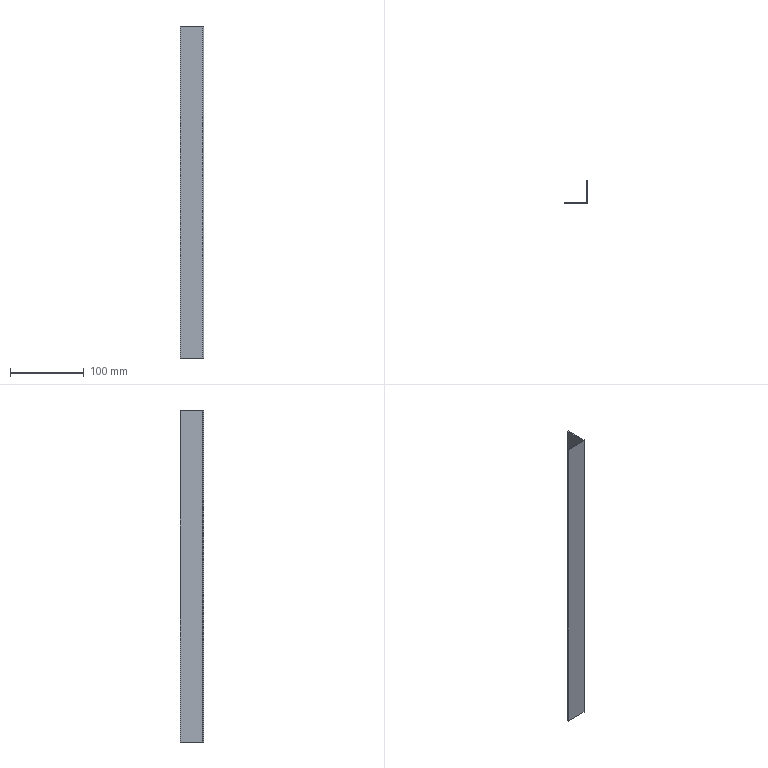Part | SolidWorks | features SplitBody 1 | 1 solid | 14 faces | box 31.5 x 31.5 x 450 mm | volume 41266 mm3 | plane 12 | cylinder 2 | commonest cylinder face diameters 0.2 x1 3.2 x1
STEP:
#1=CARTESIAN_POINT('',(-25.,30.1,185.));
#2=VERTEX_POINT('',#1);
#3=CARTESIAN_POINT('',(-23.5,30.1,185.));
#4=VERTEX_POINT('',#3);
#5=CARTESIAN_POINT('',(-25.,30.1,185.));
#6=DIRECTION('',(1.,0.,0.));
#7=VECTOR('',#6,1000.);
#8=LINE('',#5,#7);
#9=EDGE_CURVE('',#2,#4,#8,.T.);
#10=ORIENTED_EDGE('',*,*,#9,.F.);
#11=CARTESIAN_POINT('',(-25.1,30.,185.));
#12=VERTEX_POINT('',#11);
#13=CARTESIAN_POINT('',(-25.1,30.1,185.));
#14=DIRECTION('',(0.,0.,1.));
#15=DIRECTION('',(0.,1.,0.));
#16=AXIS2_PLACEMENT_3D('',#13,#14,#15);
#17=CIRCLE('',#16,0.1);
#18=EDGE_CURVE('',#12,#2,#17,.T.);
#19=ORIENTED_EDGE('',*,*,#18,.F.);
#20=CARTESIAN_POINT('',(-25.1,28.5,185.));
#21=VERTEX_POINT('',#20);
#22=CARTESIAN_POINT('',(-25.1,28.5,185.));
#23=DIRECTION('',(0.,1.,0.));
#24=VECTOR('',#23,1000.);
#25=LINE('',#22,#24);
#26=EDGE_CURVE('',#21,#12,#25,.T.);
#27=ORIENTED_EDGE('',*,*,#26,.F.);
#28=CARTESIAN_POINT('',(-25.1,30.1,185.));
#29=DIRECTION('',(0.,0.,1.));
#30=DIRECTION('',(-1.,0.,0.));
#31=AXIS2_PLACEMENT_3D('',#28,#29,#30);
#32=CIRCLE('',#31,1.6);
#33=EDGE_CURVE('',#21,#4,#32,.T.);
#34=ORIENTED_EDGE('',*,*,#33,.T.);
#35=EDGE_LOOP('',(#10,#19,#27,#34));
#36=FACE_OUTER_BOUND('',#35,.T.);
#37=CARTESIAN_POINT('',(-25.,30.1,185.));
#38=DIRECTION('',(0.,0.,1.));
#39=DIRECTION('',(0.,-1.,0.));
#40=AXIS2_PLACEMENT_3D('',#37,#38,#39);
#41=PLANE('',#40);
#42=ADVANCED_FACE('',(#36),#41,.T.);
#43=CARTESIAN_POINT('',(-25.,60.,185.));
#44=VERTEX_POINT('',#43);
#45=CARTESIAN_POINT('',(-25.,30.,185.));
#46=DIRECTION('',(0.,1.,0.));
#47=VECTOR('',#46,1000.);
#48=LINE('',#45,#47);
#49=EDGE_CURVE('',#2,#44,#48,.T.);
#50=ORIENTED_EDGE('',*,*,#49,.F.);
#51=ORIENTED_EDGE('',*,*,#9,.T.);
#52=CARTESIAN_POINT('',(-23.5,60.,185.));
#53=VERTEX_POINT('',#52);
#54=CARTESIAN_POINT('',(-23.5,30.,185.));
#55=DIRECTION('',(0.,1.,0.));
#56=VECTOR('',#55,1000.);
#57=LINE('',#54,#56);
#58=EDGE_CURVE('',#4,#53,#57,.T.);
#59=ORIENTED_EDGE('',*,*,#58,.T.);
#60=CARTESIAN_POINT('',(-23.5,60.,185.));
#61=DIRECTION('',(-1.,0.,0.));
#62=VECTOR('',#61,1000.);
#63=LINE('',#60,#62);
#64=EDGE_CURVE('',#53,#44,#63,.T.);
#65=ORIENTED_EDGE('',*,*,#64,.T.);
#66=EDGE_LOOP('',(#50,#51,#59,#65));
#67=FACE_OUTER_BOUND('',#66,.T.);
#68=CARTESIAN_POINT('',(-25.1,28.5,185.));
#69=DIRECTION('',(0.,0.,1.));
#70=DIRECTION('',(0.,-1.,0.));
#71=AXIS2_PLACEMENT_3D('',#68,#69,#70);
#72=PLANE('',#71);
#73=ADVANCED_FACE('',(#67),#72,.T.);
#74=CARTESIAN_POINT('',(-25.,60.,-265.));
#75=VERTEX_POINT('',#74);
#76=CARTESIAN_POINT('',(-25.,30.1,-265.));
#77=VERTEX_POINT('',#76);
#78=CARTESIAN_POINT('',(-25.,30.,-265.));
#79=DIRECTION('',(0.,-1.,0.));
#80=VECTOR('',#79,1000.);
#81=LINE('',#78,#80);
#82=EDGE_CURVE('',#75,#77,#81,.T.);
#83=ORIENTED_EDGE('',*,*,#82,.T.);
#84=CARTESIAN_POINT('',(-25.,30.1,-309.548));
#85=DIRECTION('',(0.,0.,1.));
#86=VECTOR('',#85,1000.);
#87=LINE('',#84,#86);
#88=EDGE_CURVE('',#77,#2,#87,.T.);
#89=ORIENTED_EDGE('',*,*,#88,.T.);
#90=ORIENTED_EDGE('',*,*,#49,.T.);
#91=CARTESIAN_POINT('',(-25.,60.,-309.548));
#92=DIRECTION('',(0.,0.,1.));
#93=VECTOR('',#92,1000.);
#94=LINE('',#91,#93);
#95=EDGE_CURVE('',#75,#44,#94,.T.);
#96=ORIENTED_EDGE('',*,*,#95,.F.);
#97=EDGE_LOOP('',(#83,#89,#90,#96));
#98=FACE_OUTER_BOUND('',#97,.T.);
#99=CARTESIAN_POINT('',(-25.,30.,-309.548));
#100=DIRECTION('',(1.,0.,0.));
#101=DIRECTION('',(0.,0.,-1.));
#102=AXIS2_PLACEMENT_3D('',#99,#100,#101);
#103=PLANE('',#102);
#104=ADVANCED_FACE('',(#98),#103,.F.);
#105=CARTESIAN_POINT('',(-23.5,60.,-265.));
#106=VERTEX_POINT('',#105);
#107=CARTESIAN_POINT('',(-23.5,60.,-309.548));
#108=DIRECTION('',(0.,0.,1.));
#109=VECTOR('',#108,1000.);
#110=LINE('',#107,#109);
#111=EDGE_CURVE('',#106,#53,#110,.T.);
#112=ORIENTED_EDGE('',*,*,#111,.F.);
#113=CARTESIAN_POINT('',(-25.,60.,-265.));
#114=DIRECTION('',(1.,0.,0.));
#115=VECTOR('',#114,1000.);
#116=LINE('',#113,#115);
#117=EDGE_CURVE('',#75,#106,#116,.T.);
#118=ORIENTED_EDGE('',*,*,#117,.F.);
#119=ORIENTED_EDGE('',*,*,#95,.T.);
#120=ORIENTED_EDGE('',*,*,#64,.F.);
#121=EDGE_LOOP('',(#112,#118,#119,#120));
#122=FACE_OUTER_BOUND('',#121,.T.);
#123=CARTESIAN_POINT('',(-23.5,60.,-309.548));
#124=DIRECTION('',(0.,1.,0.));
#125=DIRECTION('',(0.,0.,1.));
#126=AXIS2_PLACEMENT_3D('',#123,#124,#125);
#127=PLANE('',#126);
#128=ADVANCED_FACE('',(#122),#127,.T.);
#129=CARTESIAN_POINT('',(-23.5,30.1,-265.));
#130=VERTEX_POINT('',#129);
#131=CARTESIAN_POINT('',(-23.5,30.1,-309.548));
#132=DIRECTION('',(0.,0.,1.));
#133=VECTOR('',#132,1000.);
#134=LINE('',#131,#133);
#135=EDGE_CURVE('',#130,#4,#134,.T.);
#136=ORIENTED_EDGE('',*,*,#135,.F.);
#137=CARTESIAN_POINT('',(-23.5,30.,-265.));
#138=DIRECTION('',(0.,-1.,0.));
#139=VECTOR('',#138,1000.);
#140=LINE('',#137,#139);
#141=EDGE_CURVE('',#106,#130,#140,.T.);
#142=ORIENTED_EDGE('',*,*,#141,.F.);
#143=ORIENTED_EDGE('',*,*,#111,.T.);
#144=ORIENTED_EDGE('',*,*,#58,.F.);
#145=EDGE_LOOP('',(#136,#142,#143,#144));
#146=FACE_OUTER_BOUND('',#145,.T.);
#147=CARTESIAN_POINT('',(-23.5,30.,-309.548));
#148=DIRECTION('',(1.,0.,0.));
#149=DIRECTION('',(0.,0.,-1.));
#150=AXIS2_PLACEMENT_3D('',#147,#148,#149);
#151=PLANE('',#150);
#152=ADVANCED_FACE('',(#146),#151,.T.);
#153=CARTESIAN_POINT('',(-25.1,28.5,-265.));
#154=VERTEX_POINT('',#153);
#155=CARTESIAN_POINT('',(-25.1,28.5,-309.548));
#156=DIRECTION('',(0.,0.,1.));
#157=VECTOR('',#156,1000.);
#158=LINE('',#155,#157);
#159=EDGE_CURVE('',#154,#21,#158,.T.);
#160=ORIENTED_EDGE('',*,*,#159,.F.);
#161=CARTESIAN_POINT('',(-25.1,30.1,-265.));
#162=DIRECTION('',(0.,0.,-1.));
#163=DIRECTION('',(-1.,0.,0.));
#164=AXIS2_PLACEMENT_3D('',#161,#162,#163);
#165=CIRCLE('',#164,1.6);
#166=EDGE_CURVE('',#130,#154,#165,.T.);
#167=ORIENTED_EDGE('',*,*,#166,.F.);
#168=ORIENTED_EDGE('',*,*,#135,.T.);
#169=ORIENTED_EDGE('',*,*,#33,.F.);
#170=EDGE_LOOP('',(#160,#167,#168,#169));
#171=FACE_OUTER_BOUND('',#170,.T.);
#172=CARTESIAN_POINT('',(-25.1,30.1,-309.548));
#173=DIRECTION('',(0.,0.,1.));
#174=DIRECTION('',(0.,-1.,0.));
#175=AXIS2_PLACEMENT_3D('',#172,#173,#174);
#176=CYLINDRICAL_SURFACE('',#175,1.6);
#177=ADVANCED_FACE('',(#171),#176,.T.);
#178=CARTESIAN_POINT('',(-55.,28.5,-265.));
#179=VERTEX_POINT('',#178);
#180=CARTESIAN_POINT('',(-55.,28.5,185.));
#181=VERTEX_POINT('',#180);
#182=CARTESIAN_POINT('',(-55.,28.5,-309.548));
#183=DIRECTION('',(0.,0.,1.));
#184=VECTOR('',#183,1000.);
#185=LINE('',#182,#184);
#186=EDGE_CURVE('',#179,#181,#185,.T.);
#187=ORIENTED_EDGE('',*,*,#186,.F.);
#188=CARTESIAN_POINT('',(-55.,28.5,-265.));
#189=DIRECTION('',(-1.,0.,0.));
#190=VECTOR('',#189,1000.);
#191=LINE('',#188,#190);
#192=EDGE_CURVE('',#154,#179,#191,.T.);
#193=ORIENTED_EDGE('',*,*,#192,.F.);
#194=ORIENTED_EDGE('',*,*,#159,.T.);
#195=CARTESIAN_POINT('',(-55.,28.5,185.));
#196=DIRECTION('',(1.,0.,0.));
#197=VECTOR('',#196,1000.);
#198=LINE('',#195,#197);
#199=EDGE_CURVE('',#181,#21,#198,.T.);
#200=ORIENTED_EDGE('',*,*,#199,.F.);
#201=EDGE_LOOP('',(#187,#193,#194,#200));
#202=FACE_OUTER_BOUND('',#201,.T.);
#203=CARTESIAN_POINT('',(-55.,28.5,-309.548));
#204=DIRECTION('',(0.,-1.,0.));
#205=DIRECTION('',(0.,0.,-1.));
#206=AXIS2_PLACEMENT_3D('',#203,#204,#205);
#207=PLANE('',#206);
#208=ADVANCED_FACE('',(#202),#207,.T.);
#209=CARTESIAN_POINT('',(-55.,30.,-265.));
#210=VERTEX_POINT('',#209);
#211=CARTESIAN_POINT('',(-55.,30.,185.));
#212=VERTEX_POINT('',#211);
#213=CARTESIAN_POINT('',(-55.,30.,-309.548));
#214=DIRECTION('',(0.,0.,1.));
#215=VECTOR('',#214,1000.);
#216=LINE('',#213,#215);
#217=EDGE_CURVE('',#210,#212,#216,.T.);
#218=ORIENTED_EDGE('',*,*,#217,.F.);
#219=CARTESIAN_POINT('',(-55.,30.,-265.));
#220=DIRECTION('',(0.,-1.,0.));
#221=VECTOR('',#220,1000.);
#222=LINE('',#219,#221);
#223=EDGE_CURVE('',#210,#179,#222,.T.);
#224=ORIENTED_EDGE('',*,*,#223,.T.);
#225=ORIENTED_EDGE('',*,*,#186,.T.);
#226=CARTESIAN_POINT('',(-55.,30.,185.));
#227=DIRECTION('',(0.,-1.,0.));
#228=VECTOR('',#227,1000.);
#229=LINE('',#226,#228);
#230=EDGE_CURVE('',#212,#181,#229,.T.);
#231=ORIENTED_EDGE('',*,*,#230,.F.);
#232=EDGE_LOOP('',(#218,#224,#225,#231));
#233=FACE_OUTER_BOUND('',#232,.T.);
#234=CARTESIAN_POINT('',(-55.,30.,-309.548));
#235=DIRECTION('',(-1.,0.,0.));
#236=DIRECTION('',(0.,0.,1.));
#237=AXIS2_PLACEMENT_3D('',#234,#235,#236);
#238=PLANE('',#237);
#239=ADVANCED_FACE('',(#233),#238,.T.);
#240=CARTESIAN_POINT('',(-25.1,30.,-265.));
#241=VERTEX_POINT('',#240);
#242=CARTESIAN_POINT('',(-55.,30.,-265.));
#243=DIRECTION('',(-1.,0.,0.));
#244=VECTOR('',#243,1000.);
#245=LINE('',#242,#244);
#246=EDGE_CURVE('',#241,#210,#245,.T.);
#247=ORIENTED_EDGE('',*,*,#246,.T.);
#248=ORIENTED_EDGE('',*,*,#217,.T.);
#249=CARTESIAN_POINT('',(-55.,30.,185.));
#250=DIRECTION('',(1.,0.,0.));
#251=VECTOR('',#250,1000.);
#252=LINE('',#249,#251);
#253=EDGE_CURVE('',#212,#12,#252,.T.);
#254=ORIENTED_EDGE('',*,*,#253,.T.);
#255=CARTESIAN_POINT('',(-25.1,30.,-309.548));
#256=DIRECTION('',(0.,0.,1.));
#257=VECTOR('',#256,1000.);
#258=LINE('',#255,#257);
#259=EDGE_CURVE('',#241,#12,#258,.T.);
#260=ORIENTED_EDGE('',*,*,#259,.F.);
#261=EDGE_LOOP('',(#247,#248,#254,#260));
#262=FACE_OUTER_BOUND('',#261,.T.);
#263=CARTESIAN_POINT('',(-55.,30.,-309.548));
#264=DIRECTION('',(0.,-1.,0.));
#265=DIRECTION('',(0.,0.,-1.));
#266=AXIS2_PLACEMENT_3D('',#263,#264,#265);
#267=PLANE('',#266);
#268=ADVANCED_FACE('',(#262),#267,.F.);
#269=CARTESIAN_POINT('',(-25.1,30.1,-265.));
#270=DIRECTION('',(0.,0.,-1.));
#271=DIRECTION('',(1.,0.,0.));
#272=AXIS2_PLACEMENT_3D('',#269,#270,#271);
#273=CIRCLE('',#272,0.1);
#274=EDGE_CURVE('',#77,#241,#273,.T.);
#275=ORIENTED_EDGE('',*,*,#274,.T.);
#276=ORIENTED_EDGE('',*,*,#259,.T.);
#277=ORIENTED_EDGE('',*,*,#18,.T.);
#278=ORIENTED_EDGE('',*,*,#88,.F.);
#279=EDGE_LOOP('',(#275,#276,#277,#278));
#280=FACE_OUTER_BOUND('',#279,.T.);
#281=CARTESIAN_POINT('',(-25.1,30.1,-309.548));
#282=DIRECTION('',(0.,0.,1.));
#283=DIRECTION('',(0.,-1.,0.));
#284=AXIS2_PLACEMENT_3D('',#281,#282,#283);
#285=CYLINDRICAL_SURFACE('',#284,0.1);
#286=ADVANCED_FACE('',(#280),#285,.F.);
#287=ORIENTED_EDGE('',*,*,#199,.T.);
#288=ORIENTED_EDGE('',*,*,#26,.T.);
#289=ORIENTED_EDGE('',*,*,#253,.F.);
#290=ORIENTED_EDGE('',*,*,#230,.T.);
#291=EDGE_LOOP('',(#287,#288,#289,#290));
#292=FACE_OUTER_BOUND('',#291,.T.);
#293=CARTESIAN_POINT('',(-25.1,30.1,185.));
#294=DIRECTION('',(0.,0.,-1.));
#295=DIRECTION('',(-1.,0.,0.));
#296=AXIS2_PLACEMENT_3D('',#293,#294,#295);
#297=PLANE('',#296);
#298=ADVANCED_FACE('',(#292),#297,.F.);
#299=CARTESIAN_POINT('',(-25.,30.1,-265.));
#300=DIRECTION('',(1.,0.,0.));
#301=VECTOR('',#300,1000.);
#302=LINE('',#299,#301);
#303=EDGE_CURVE('',#77,#130,#302,.T.);
#304=ORIENTED_EDGE('',*,*,#303,.F.);
#305=ORIENTED_EDGE('',*,*,#82,.F.);
#306=ORIENTED_EDGE('',*,*,#117,.T.);
#307=ORIENTED_EDGE('',*,*,#141,.T.);
#308=EDGE_LOOP('',(#304,#305,#306,#307));
#309=FACE_OUTER_BOUND('',#308,.T.);
#310=CARTESIAN_POINT('',(-25.,30.,-265.));
#311=DIRECTION('',(0.,0.,1.));
#312=DIRECTION('',(0.,-1.,0.));
#313=AXIS2_PLACEMENT_3D('',#310,#311,#312);
#314=PLANE('',#313);
#315=ADVANCED_FACE('',(#309),#314,.F.);
#316=ORIENTED_EDGE('',*,*,#223,.F.);
#317=ORIENTED_EDGE('',*,*,#246,.F.);
#318=CARTESIAN_POINT('',(-25.1,30.,-265.));
#319=DIRECTION('',(0.,-1.,0.));
#320=VECTOR('',#319,1000.);
#321=LINE('',#318,#320);
#322=EDGE_CURVE('',#241,#154,#321,.T.);
#323=ORIENTED_EDGE('',*,*,#322,.T.);
#324=ORIENTED_EDGE('',*,*,#192,.T.);
#325=EDGE_LOOP('',(#316,#317,#323,#324));
#326=FACE_OUTER_BOUND('',#325,.T.);
#327=CARTESIAN_POINT('',(-55.,30.,-265.));
#328=DIRECTION('',(0.,0.,1.));
#329=DIRECTION('',(-1.,0.,0.));
#330=AXIS2_PLACEMENT_3D('',#327,#328,#329);
#331=PLANE('',#330);
#332=ADVANCED_FACE('',(#326),#331,.F.);
#333=ORIENTED_EDGE('',*,*,#166,.T.);
#334=ORIENTED_EDGE('',*,*,#322,.F.);
#335=ORIENTED_EDGE('',*,*,#274,.F.);
#336=ORIENTED_EDGE('',*,*,#303,.T.);
#337=EDGE_LOOP('',(#333,#334,#335,#336));
#338=FACE_OUTER_BOUND('',#337,.T.);
#339=CARTESIAN_POINT('',(-25.1,30.1,-265.));
#340=DIRECTION('',(0.,0.,-1.));
#341=DIRECTION('',(-1.,0.,0.));
#342=AXIS2_PLACEMENT_3D('',#339,#340,#341);
#343=PLANE('',#342);
#344=ADVANCED_FACE('',(#338),#343,.T.);
#345=CLOSED_SHELL('',(#42,#73,#104,#128,#152,#177,#208,#239,#268,#286,#298,#315,#332,#344));
#346=MANIFOLD_SOLID_BREP('',#345);
#347=CARTESIAN_POINT('',(0.,0.,0.));
#348=DIRECTION('',(0.,0.,1.));
#349=DIRECTION('',(1.,0.,0.));
#350=AXIS2_PLACEMENT_3D('',#347,#348,#349);
#351=(LENGTH_UNIT()NAMED_UNIT(*)SI_UNIT(.MILLI.,.METRE.));
#352=UNCERTAINTY_MEASURE_WITH_UNIT(LENGTH_MEASURE(0.00001),#351,'','');
#353=(NAMED_UNIT(*)PLANE_ANGLE_UNIT()SI_UNIT($,.RADIAN.));
#354=(NAMED_UNIT(*)SI_UNIT($,.STERADIAN.)SOLID_ANGLE_UNIT());
#355=(GEOMETRIC_REPRESENTATION_CONTEXT(3)GLOBAL_UNCERTAINTY_ASSIGNED_CONTEXT((#352))GLOBAL_UNIT_ASSIGNED_CONTEXT((#351,#353,#354))REPRESENTATION_CONTEXT('',''));
#356=ADVANCED_BREP_SHAPE_REPRESENTATION('',(#346,#350),#355);